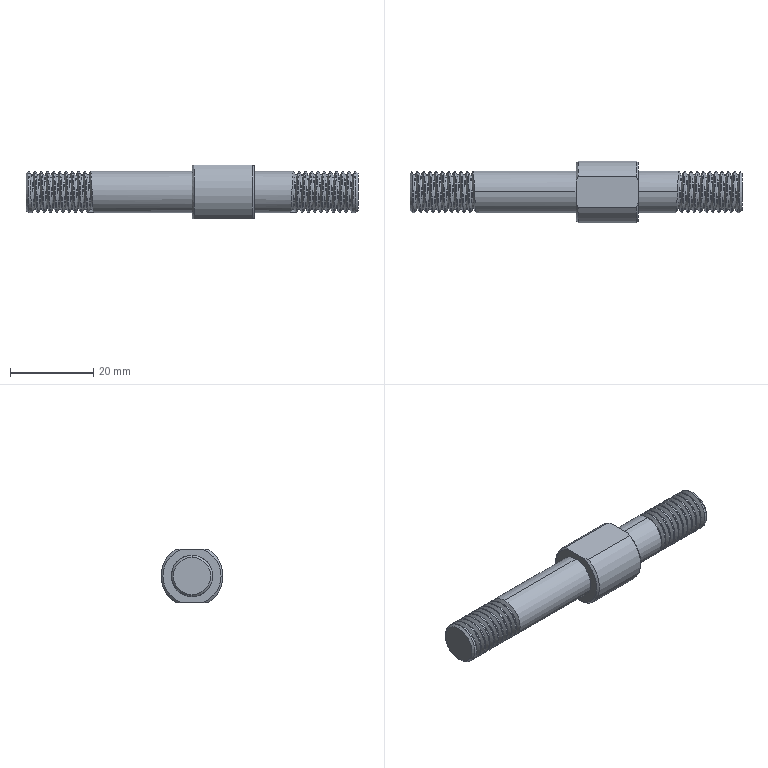Part | SolidWorks | features Chamfer 1, ICE 1, MirrorPattern 1, Revolution 1, SweepThread 1 | 1 solid | 70 faces | box 80 x 15 x 13 mm | volume 7147 mm3 | cylinder 46 | plane 10 | cone 8 | spline 6 | commonest cylinder face diameters 10 x44 15 x2